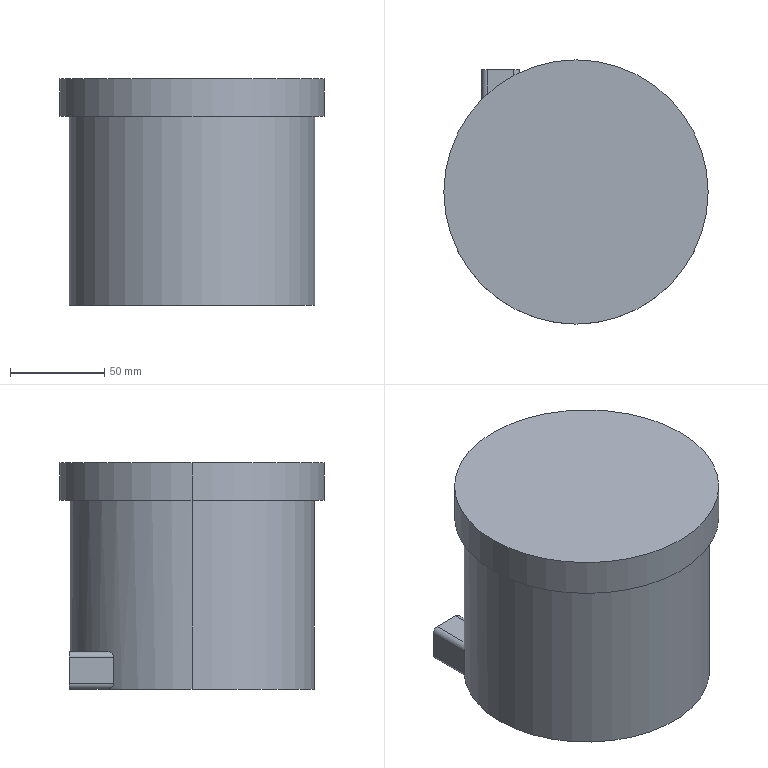Part | SolidWorks | features ICE 3, Extrusion 1, Fillet 1 | 1 solid | 18 faces | box 140 x 140 x 120 mm | volume 1639624 mm3 | cylinder 10 | plane 8 | commonest cylinder face diameters 6 x4 10 x2 130 x2 140 x2
STEP:
#1=CARTESIAN_POINT('',(-40.,50.,5.));
#2=VERTEX_POINT('',#1);
#3=CARTESIAN_POINT('',(-40.,50.,15.));
#4=VERTEX_POINT('',#3);
#5=CARTESIAN_POINT('',(-40.,50.,10.));
#6=DIRECTION('',(0.,1.,0.));
#7=DIRECTION('',(0.,0.,1.));
#8=AXIS2_PLACEMENT_3D('',#5,#6,#7);
#9=CIRCLE('',#8,5.);
#10=EDGE_CURVE('',#2,#4,#9,.T.);
#11=ORIENTED_EDGE('',*,*,#10,.F.);
#12=CARTESIAN_POINT('',(-40.,65.,5.));
#13=VERTEX_POINT('',#12);
#14=CARTESIAN_POINT('',(-40.,50.,5.));
#15=DIRECTION('',(0.,1.,0.));
#16=VECTOR('',#15,1000.);
#17=LINE('',#14,#16);
#18=EDGE_CURVE('',#2,#13,#17,.T.);
#19=ORIENTED_EDGE('',*,*,#18,.T.);
#20=CARTESIAN_POINT('',(-40.,65.,15.));
#21=VERTEX_POINT('',#20);
#22=CARTESIAN_POINT('',(-40.,65.,10.));
#23=DIRECTION('',(0.,1.,0.));
#24=DIRECTION('',(0.,0.,1.));
#25=AXIS2_PLACEMENT_3D('',#22,#23,#24);
#26=CIRCLE('',#25,5.);
#27=EDGE_CURVE('',#13,#21,#26,.T.);
#28=ORIENTED_EDGE('',*,*,#27,.T.);
#29=CARTESIAN_POINT('',(-40.,50.,15.));
#30=DIRECTION('',(0.,1.,0.));
#31=VECTOR('',#30,1000.);
#32=LINE('',#29,#31);
#33=EDGE_CURVE('',#4,#21,#32,.T.);
#34=ORIENTED_EDGE('',*,*,#33,.F.);
#35=EDGE_LOOP('',(#11,#19,#28,#34));
#36=FACE_OUTER_BOUND('',#35,.T.);
#37=CARTESIAN_POINT('',(-40.,50.,10.));
#38=DIRECTION('',(0.,1.,0.));
#39=DIRECTION('',(0.,0.,1.));
#40=AXIS2_PLACEMENT_3D('',#37,#38,#39);
#41=CYLINDRICAL_SURFACE('',#40,5.);
#42=ADVANCED_FACE('',(#36),#41,.F.);
#43=CARTESIAN_POINT('',(70.,0.,120.));
#44=VERTEX_POINT('',#43);
#45=CARTESIAN_POINT('',(-70.,0.,120.));
#46=VERTEX_POINT('',#45);
#47=CARTESIAN_POINT('',(0.,0.,120.));
#48=DIRECTION('',(0.,0.,1.));
#49=DIRECTION('',(1.,0.,0.));
#50=AXIS2_PLACEMENT_3D('',#47,#48,#49);
#51=CIRCLE('',#50,70.);
#52=EDGE_CURVE('',#44,#46,#51,.T.);
#53=ORIENTED_EDGE('',*,*,#52,.F.);
#54=CARTESIAN_POINT('',(70.,0.,100.));
#55=VERTEX_POINT('',#54);
#56=CARTESIAN_POINT('',(70.,0.,120.));
#57=DIRECTION('',(0.,0.,-1.));
#58=VECTOR('',#57,1000.);
#59=LINE('',#56,#58);
#60=EDGE_CURVE('',#44,#55,#59,.T.);
#61=ORIENTED_EDGE('',*,*,#60,.T.);
#62=CARTESIAN_POINT('',(-70.,0.,100.));
#63=VERTEX_POINT('',#62);
#64=CARTESIAN_POINT('',(0.,0.,100.));
#65=DIRECTION('',(0.,0.,1.));
#66=DIRECTION('',(1.,0.,0.));
#67=AXIS2_PLACEMENT_3D('',#64,#65,#66);
#68=CIRCLE('',#67,70.);
#69=EDGE_CURVE('',#55,#63,#68,.T.);
#70=ORIENTED_EDGE('',*,*,#69,.T.);
#71=CARTESIAN_POINT('',(-70.,0.,120.));
#72=DIRECTION('',(0.,0.,-1.));
#73=VECTOR('',#72,1000.);
#74=LINE('',#71,#73);
#75=EDGE_CURVE('',#46,#63,#74,.T.);
#76=ORIENTED_EDGE('',*,*,#75,.F.);
#77=EDGE_LOOP('',(#53,#61,#70,#76));
#78=FACE_OUTER_BOUND('',#77,.T.);
#79=CARTESIAN_POINT('',(0.,0.,120.));
#80=DIRECTION('',(0.,0.,-1.));
#81=DIRECTION('',(-1.,0.,0.));
#82=AXIS2_PLACEMENT_3D('',#79,#80,#81);
#83=CYLINDRICAL_SURFACE('',#82,70.);
#84=ADVANCED_FACE('',(#78),#83,.T.);
#85=CARTESIAN_POINT('',(65.,0.,100.));
#86=VERTEX_POINT('',#85);
#87=CARTESIAN_POINT('',(-65.,0.,100.));
#88=VERTEX_POINT('',#87);
#89=CARTESIAN_POINT('',(0.,0.,100.));
#90=DIRECTION('',(0.,0.,1.));
#91=DIRECTION('',(1.,0.,0.));
#92=AXIS2_PLACEMENT_3D('',#89,#90,#91);
#93=CIRCLE('',#92,65.);
#94=EDGE_CURVE('',#86,#88,#93,.T.);
#95=ORIENTED_EDGE('',*,*,#94,.F.);
#96=CARTESIAN_POINT('',(65.,0.,0.));
#97=VERTEX_POINT('',#96);
#98=CARTESIAN_POINT('',(65.,0.,100.));
#99=DIRECTION('',(0.,0.,-1.));
#100=VECTOR('',#99,1000.);
#101=LINE('',#98,#100);
#102=EDGE_CURVE('',#86,#97,#101,.T.);
#103=ORIENTED_EDGE('',*,*,#102,.T.);
#104=CARTESIAN_POINT('',(-33.,56.,0.));
#105=VERTEX_POINT('',#104);
#106=CARTESIAN_POINT('',(0.,0.,0.));
#107=DIRECTION('',(0.,0.,1.));
#108=DIRECTION('',(1.,0.,0.));
#109=AXIS2_PLACEMENT_3D('',#106,#107,#108);
#110=CIRCLE('',#109,65.);
#111=EDGE_CURVE('',#97,#105,#110,.T.);
#112=ORIENTED_EDGE('',*,*,#111,.T.);
#113=CARTESIAN_POINT('',(-30.,57.663,3.));
#114=VERTEX_POINT('',#113);
#115=CARTESIAN_POINT('',(-33.,56.,0.));
#116=CARTESIAN_POINT('',(-32.633,56.216,0.));
#117=CARTESIAN_POINT('',(-32.275,56.422,0.06519));
#118=CARTESIAN_POINT('',(-31.753,56.717,0.2653));
#119=CARTESIAN_POINT('',(-31.58,56.813,0.3504));
#120=CARTESIAN_POINT('',(-31.256,56.992,0.5513));
#121=CARTESIAN_POINT('',(-31.103,57.075,0.6674));
#122=CARTESIAN_POINT('',(-30.816,57.231,0.9335));
#123=CARTESIAN_POINT('',(-30.681,57.303,1.086));
#124=CARTESIAN_POINT('',(-30.447,57.428,1.412));
#125=CARTESIAN_POINT('',(-30.345,57.482,1.588));
#126=CARTESIAN_POINT('',(-30.176,57.571,1.966));
#127=CARTESIAN_POINT('',(-30.11,57.605,2.168));
#128=CARTESIAN_POINT('',(-30.023,57.651,2.577));
#129=CARTESIAN_POINT('',(-30.,57.663,2.786));
#130=CARTESIAN_POINT('',(-30.,57.663,3.));
#131=B_SPLINE_CURVE_WITH_KNOTS('',3,(#115,#116,#117,#118,#119,#120,#121,#122,#123,#124,#125,#126,#127,#128,#129,#130),.UNSPECIFIED.,.F.,.F.,(4,2,2,2,2,2,2,4),(0.,0.001254,0.001881,0.002508,0.003135,0.003762,0.004389,0.005016),.UNSPECIFIED.);
#132=EDGE_CURVE('',#105,#114,#131,.T.);
#133=ORIENTED_EDGE('',*,*,#132,.T.);
#134=CARTESIAN_POINT('',(-30.,57.663,17.));
#135=VERTEX_POINT('',#134);
#136=CARTESIAN_POINT('',(-30.,57.663,100.));
#137=DIRECTION('',(0.,0.,1.));
#138=VECTOR('',#137,1000.);
#139=LINE('',#136,#138);
#140=EDGE_CURVE('',#114,#135,#139,.T.);
#141=ORIENTED_EDGE('',*,*,#140,.T.);
#142=CARTESIAN_POINT('',(-33.,56.,20.));
#143=VERTEX_POINT('',#142);
#144=CARTESIAN_POINT('',(-30.,57.663,17.));
#145=CARTESIAN_POINT('',(-30.,57.663,17.213));
#146=CARTESIAN_POINT('',(-30.022,57.651,17.422));
#147=CARTESIAN_POINT('',(-30.11,57.606,17.83));
#148=CARTESIAN_POINT('',(-30.176,57.571,18.032));
#149=CARTESIAN_POINT('',(-30.343,57.483,18.408));
#150=CARTESIAN_POINT('',(-30.445,57.429,18.585));
#151=CARTESIAN_POINT('',(-30.681,57.303,18.914));
#152=CARTESIAN_POINT('',(-30.813,57.233,19.063));
#153=CARTESIAN_POINT('',(-31.099,57.078,19.329));
#154=CARTESIAN_POINT('',(-31.256,56.992,19.448));
#155=CARTESIAN_POINT('',(-31.579,56.814,19.649));
#156=CARTESIAN_POINT('',(-31.748,56.72,19.733));
#157=CARTESIAN_POINT('',(-32.098,56.522,19.867));
#158=CARTESIAN_POINT('',(-32.277,56.42,19.917));
#159=CARTESIAN_POINT('',(-32.636,56.213,19.983));
#160=CARTESIAN_POINT('',(-32.817,56.108,20.));
#161=CARTESIAN_POINT('',(-33.,56.,20.));
#162=B_SPLINE_CURVE_WITH_KNOTS('',3,(#144,#145,#146,#147,#148,#149,#150,#151,#152,#153,#154,#155,#156,#157,#158,#159,#160,#161),.UNSPECIFIED.,.F.,.F.,(4,2,2,2,2,2,2,2,4),(0.,0.0006295,0.001259,0.001888,0.002518,0.003147,0.003777,0.004406,0.005036),.UNSPECIFIED.);
#163=EDGE_CURVE('',#135,#143,#162,.T.);
#164=ORIENTED_EDGE('',*,*,#163,.T.);
#165=CARTESIAN_POINT('',(-47.,44.9,20.));
#166=VERTEX_POINT('',#165);
#167=CARTESIAN_POINT('',(0.,0.,20.));
#168=DIRECTION('',(0.,0.,1.));
#169=DIRECTION('',(1.,0.,0.));
#170=AXIS2_PLACEMENT_3D('',#167,#168,#169);
#171=CIRCLE('',#170,65.);
#172=EDGE_CURVE('',#143,#166,#171,.T.);
#173=ORIENTED_EDGE('',*,*,#172,.T.);
#174=CARTESIAN_POINT('',(-50.,41.533,17.));
#175=VERTEX_POINT('',#174);
#176=CARTESIAN_POINT('',(-47.,44.9,20.));
#177=CARTESIAN_POINT('',(-47.344,44.54,20.));
#178=CARTESIAN_POINT('',(-47.677,44.183,19.943));
#179=CARTESIAN_POINT('',(-48.322,43.477,19.715));
#180=CARTESIAN_POINT('',(-48.636,43.124,19.542));
#181=CARTESIAN_POINT('',(-49.063,42.636,19.186));
#182=CARTESIAN_POINT('',(-49.2,42.478,19.049));
#183=CARTESIAN_POINT('',(-49.453,42.183,18.738));
#184=CARTESIAN_POINT('',(-49.568,42.048,18.566));
#185=CARTESIAN_POINT('',(-49.768,41.811,18.177));
#186=CARTESIAN_POINT('',(-49.852,41.711,17.962));
#187=CARTESIAN_POINT('',(-49.939,41.607,17.615));
#188=CARTESIAN_POINT('',(-49.962,41.579,17.494));
#189=CARTESIAN_POINT('',(-49.992,41.543,17.249));
#190=CARTESIAN_POINT('',(-50.,41.533,17.126));
#191=CARTESIAN_POINT('',(-50.,41.533,17.));
#192=B_SPLINE_CURVE_WITH_KNOTS('',3,(#176,#177,#178,#179,#180,#181,#182,#183,#184,#185,#186,#187,#188,#189,#190,#191),.UNSPECIFIED.,.F.,.F.,(4,2,2,2,2,2,2,4),(0.,0.001472,0.002944,0.00368,0.004416,0.005152,0.00552,0.005888),.UNSPECIFIED.);
#193=EDGE_CURVE('',#166,#175,#192,.T.);
#194=ORIENTED_EDGE('',*,*,#193,.T.);
#195=CARTESIAN_POINT('',(-50.,41.533,3.));
#196=VERTEX_POINT('',#195);
#197=CARTESIAN_POINT('',(-50.,41.533,100.));
#198=DIRECTION('',(0.,0.,-1.));
#199=VECTOR('',#198,1000.);
#200=LINE('',#197,#199);
#201=EDGE_CURVE('',#175,#196,#200,.T.);
#202=ORIENTED_EDGE('',*,*,#201,.T.);
#203=CARTESIAN_POINT('',(-47.,44.9,0.));
#204=VERTEX_POINT('',#203);
#205=CARTESIAN_POINT('',(-50.,41.533,3.));
#206=CARTESIAN_POINT('',(-50.,41.533,2.749));
#207=CARTESIAN_POINT('',(-49.969,41.571,2.507));
#208=CARTESIAN_POINT('',(-49.852,41.71,2.04));
#209=CARTESIAN_POINT('',(-49.77,41.809,1.827));
#210=CARTESIAN_POINT('',(-49.569,42.046,1.436));
#211=CARTESIAN_POINT('',(-49.454,42.182,1.263));
#212=CARTESIAN_POINT('',(-49.203,42.474,0.9543));
#213=CARTESIAN_POINT('',(-49.066,42.633,0.8168));
#214=CARTESIAN_POINT('',(-48.638,43.122,0.4594));
#215=CARTESIAN_POINT('',(-48.33,43.468,0.2887));
#216=CARTESIAN_POINT('',(-47.678,44.182,0.05729));
#217=CARTESIAN_POINT('',(-47.344,44.54,0.));
#218=CARTESIAN_POINT('',(-47.,44.9,0.));
#219=B_SPLINE_CURVE_WITH_KNOTS('',3,(#205,#206,#207,#208,#209,#210,#211,#212,#213,#214,#215,#216,#217,#218),.UNSPECIFIED.,.F.,.F.,(4,2,2,2,2,2,4),(0.,0.0007398,0.00148,0.002219,0.002959,0.004439,0.005918),.UNSPECIFIED.);
#220=EDGE_CURVE('',#196,#204,#219,.T.);
#221=ORIENTED_EDGE('',*,*,#220,.T.);
#222=CARTESIAN_POINT('',(-65.,0.,0.));
#223=VERTEX_POINT('',#222);
#224=CARTESIAN_POINT('',(0.,0.,0.));
#225=DIRECTION('',(0.,0.,1.));
#226=DIRECTION('',(1.,0.,0.));
#227=AXIS2_PLACEMENT_3D('',#224,#225,#226);
#228=CIRCLE('',#227,65.);
#229=EDGE_CURVE('',#204,#223,#228,.T.);
#230=ORIENTED_EDGE('',*,*,#229,.T.);
#231=CARTESIAN_POINT('',(-65.,0.,100.));
#232=DIRECTION('',(0.,0.,-1.));
#233=VECTOR('',#232,1000.);
#234=LINE('',#231,#233);
#235=EDGE_CURVE('',#88,#223,#234,.T.);
#236=ORIENTED_EDGE('',*,*,#235,.F.);
#237=EDGE_LOOP('',(#95,#103,#112,#133,#141,#164,#173,#194,#202,#221,#230,#236));
#238=FACE_OUTER_BOUND('',#237,.T.);
#239=CARTESIAN_POINT('',(0.,0.,100.));
#240=DIRECTION('',(0.,0.,-1.));
#241=DIRECTION('',(-1.,0.,0.));
#242=AXIS2_PLACEMENT_3D('',#239,#240,#241);
#243=CYLINDRICAL_SURFACE('',#242,65.);
#244=ADVANCED_FACE('',(#238),#243,.T.);
#245=ORIENTED_EDGE('',*,*,#102,.F.);
#246=CARTESIAN_POINT('',(0.,0.,100.));
#247=DIRECTION('',(0.,0.,1.));
#248=DIRECTION('',(1.,0.,0.));
#249=AXIS2_PLACEMENT_3D('',#246,#247,#248);
#250=CIRCLE('',#249,65.);
#251=EDGE_CURVE('',#88,#86,#250,.T.);
#252=ORIENTED_EDGE('',*,*,#251,.F.);
#253=ORIENTED_EDGE('',*,*,#235,.T.);
#254=CARTESIAN_POINT('',(0.,0.,0.));
#255=DIRECTION('',(0.,0.,1.));
#256=DIRECTION('',(1.,0.,0.));
#257=AXIS2_PLACEMENT_3D('',#254,#255,#256);
#258=CIRCLE('',#257,65.);
#259=EDGE_CURVE('',#223,#97,#258,.T.);
#260=ORIENTED_EDGE('',*,*,#259,.T.);
#261=EDGE_LOOP('',(#245,#252,#253,#260));
#262=FACE_OUTER_BOUND('',#261,.T.);
#263=CARTESIAN_POINT('',(0.,0.,100.));
#264=DIRECTION('',(0.,0.,-1.));
#265=DIRECTION('',(-1.,0.,0.));
#266=AXIS2_PLACEMENT_3D('',#263,#264,#265);
#267=CYLINDRICAL_SURFACE('',#266,65.);
#268=ADVANCED_FACE('',(#262),#267,.T.);
#269=CARTESIAN_POINT('',(-47.,65.,0.));
#270=VERTEX_POINT('',#269);
#271=CARTESIAN_POINT('',(-33.,65.,0.));
#272=VERTEX_POINT('',#271);
#273=CARTESIAN_POINT('',(-30.,65.,0.));
#274=DIRECTION('',(1.,0.,0.));
#275=VECTOR('',#274,1000.);
#276=LINE('',#273,#275);
#277=EDGE_CURVE('',#270,#272,#276,.T.);
#278=ORIENTED_EDGE('',*,*,#277,.T.);
#279=CARTESIAN_POINT('',(-33.,57.663,0.));
#280=DIRECTION('',(0.,-1.,0.));
#281=VECTOR('',#280,1000.);
#282=LINE('',#279,#281);
#283=EDGE_CURVE('',#272,#105,#282,.T.);
#284=ORIENTED_EDGE('',*,*,#283,.T.);
#285=ORIENTED_EDGE('',*,*,#111,.F.);
#286=ORIENTED_EDGE('',*,*,#259,.F.);
#287=ORIENTED_EDGE('',*,*,#229,.F.);
#288=CARTESIAN_POINT('',(-47.,65.,0.));
#289=DIRECTION('',(0.,1.,0.));
#290=VECTOR('',#289,1000.);
#291=LINE('',#288,#290);
#292=EDGE_CURVE('',#204,#270,#291,.T.);
#293=ORIENTED_EDGE('',*,*,#292,.T.);
#294=EDGE_LOOP('',(#278,#284,#285,#286,#287,#293));
#295=FACE_OUTER_BOUND('',#294,.T.);
#296=CARTESIAN_POINT('',(0.,0.,0.));
#297=DIRECTION('',(0.,0.,1.));
#298=DIRECTION('',(1.,0.,0.));
#299=AXIS2_PLACEMENT_3D('',#296,#297,#298);
#300=PLANE('',#299);
#301=ADVANCED_FACE('',(#295),#300,.F.);
#302=ORIENTED_EDGE('',*,*,#60,.F.);
#303=CARTESIAN_POINT('',(0.,0.,120.));
#304=DIRECTION('',(0.,0.,1.));
#305=DIRECTION('',(1.,0.,0.));
#306=AXIS2_PLACEMENT_3D('',#303,#304,#305);
#307=CIRCLE('',#306,70.);
#308=EDGE_CURVE('',#46,#44,#307,.T.);
#309=ORIENTED_EDGE('',*,*,#308,.F.);
#310=ORIENTED_EDGE('',*,*,#75,.T.);
#311=CARTESIAN_POINT('',(0.,0.,100.));
#312=DIRECTION('',(0.,0.,1.));
#313=DIRECTION('',(1.,0.,0.));
#314=AXIS2_PLACEMENT_3D('',#311,#312,#313);
#315=CIRCLE('',#314,70.);
#316=EDGE_CURVE('',#63,#55,#315,.T.);
#317=ORIENTED_EDGE('',*,*,#316,.T.);
#318=EDGE_LOOP('',(#302,#309,#310,#317));
#319=FACE_OUTER_BOUND('',#318,.T.);
#320=CARTESIAN_POINT('',(0.,0.,120.));
#321=DIRECTION('',(0.,0.,-1.));
#322=DIRECTION('',(-1.,0.,0.));
#323=AXIS2_PLACEMENT_3D('',#320,#321,#322);
#324=CYLINDRICAL_SURFACE('',#323,70.);
#325=ADVANCED_FACE('',(#319),#324,.T.);
#326=ORIENTED_EDGE('',*,*,#308,.T.);
#327=ORIENTED_EDGE('',*,*,#52,.T.);
#328=EDGE_LOOP('',(#326,#327));
#329=FACE_OUTER_BOUND('',#328,.T.);
#330=CARTESIAN_POINT('',(0.,0.,120.));
#331=DIRECTION('',(0.,0.,1.));
#332=DIRECTION('',(1.,0.,0.));
#333=AXIS2_PLACEMENT_3D('',#330,#331,#332);
#334=PLANE('',#333);
#335=ADVANCED_FACE('',(#329),#334,.T.);
#336=ORIENTED_EDGE('',*,*,#251,.T.);
#337=ORIENTED_EDGE('',*,*,#94,.T.);
#338=EDGE_LOOP('',(#336,#337));
#339=FACE_BOUND('',#338,.T.);
#340=ORIENTED_EDGE('',*,*,#316,.F.);
#341=ORIENTED_EDGE('',*,*,#69,.F.);
#342=EDGE_LOOP('',(#340,#341));
#343=FACE_OUTER_BOUND('',#342,.T.);
#344=CARTESIAN_POINT('',(0.,0.,100.));
#345=DIRECTION('',(0.,0.,1.));
#346=DIRECTION('',(1.,0.,0.));
#347=AXIS2_PLACEMENT_3D('',#344,#345,#346);
#348=PLANE('',#347);
#349=ADVANCED_FACE('',(#339,#343),#348,.F.);
#350=ORIENTED_EDGE('',*,*,#140,.F.);
#351=CARTESIAN_POINT('',(-30.,65.,3.));
#352=VERTEX_POINT('',#351);
#353=CARTESIAN_POINT('',(-30.,65.,3.));
#354=DIRECTION('',(0.,1.,0.));
#355=VECTOR('',#354,1000.);
#356=LINE('',#353,#355);
#357=EDGE_CURVE('',#114,#352,#356,.T.);
#358=ORIENTED_EDGE('',*,*,#357,.T.);
#359=CARTESIAN_POINT('',(-30.,65.,17.));
#360=VERTEX_POINT('',#359);
#361=CARTESIAN_POINT('',(-30.,65.,20.));
#362=DIRECTION('',(0.,0.,-1.));
#363=VECTOR('',#362,1000.);
#364=LINE('',#361,#363);
#365=EDGE_CURVE('',#360,#352,#364,.T.);
#366=ORIENTED_EDGE('',*,*,#365,.F.);
#367=CARTESIAN_POINT('',(-30.,40.911,17.));
#368=DIRECTION('',(0.,-1.,0.));
#369=VECTOR('',#368,1000.);
#370=LINE('',#367,#369);
#371=EDGE_CURVE('',#360,#135,#370,.T.);
#372=ORIENTED_EDGE('',*,*,#371,.T.);
#373=EDGE_LOOP('',(#350,#358,#366,#372));
#374=FACE_OUTER_BOUND('',#373,.T.);
#375=CARTESIAN_POINT('',(-30.,40.911,20.));
#376=DIRECTION('',(1.,0.,0.));
#377=DIRECTION('',(0.,0.,-1.));
#378=AXIS2_PLACEMENT_3D('',#375,#376,#377);
#379=PLANE('',#378);
#380=ADVANCED_FACE('',(#374),#379,.T.);
#381=CARTESIAN_POINT('',(-50.,65.,17.));
#382=VERTEX_POINT('',#381);
#383=CARTESIAN_POINT('',(-50.,65.,3.));
#384=VERTEX_POINT('',#383);
#385=CARTESIAN_POINT('',(-50.,65.,20.));
#386=DIRECTION('',(0.,0.,-1.));
#387=VECTOR('',#386,1000.);
#388=LINE('',#385,#387);
#389=EDGE_CURVE('',#382,#384,#388,.T.);
#390=ORIENTED_EDGE('',*,*,#389,.T.);
#391=CARTESIAN_POINT('',(-50.,41.533,3.));
#392=DIRECTION('',(0.,-1.,0.));
#393=VECTOR('',#392,1000.);
#394=LINE('',#391,#393);
#395=EDGE_CURVE('',#384,#196,#394,.T.);
#396=ORIENTED_EDGE('',*,*,#395,.T.);
#397=ORIENTED_EDGE('',*,*,#201,.F.);
#398=CARTESIAN_POINT('',(-50.,40.911,17.));
#399=DIRECTION('',(0.,1.,0.));
#400=VECTOR('',#399,1000.);
#401=LINE('',#398,#400);
#402=EDGE_CURVE('',#175,#382,#401,.T.);
#403=ORIENTED_EDGE('',*,*,#402,.T.);
#404=EDGE_LOOP('',(#390,#396,#397,#403));
#405=FACE_OUTER_BOUND('',#404,.T.);
#406=CARTESIAN_POINT('',(-50.,40.911,20.));
#407=DIRECTION('',(-1.,0.,0.));
#408=DIRECTION('',(0.,0.,1.));
#409=AXIS2_PLACEMENT_3D('',#406,#407,#408);
#410=PLANE('',#409);
#411=ADVANCED_FACE('',(#405),#410,.T.);
#412=CARTESIAN_POINT('',(-40.,65.,10.));
#413=DIRECTION('',(0.,1.,0.));
#414=DIRECTION('',(0.,0.,1.));
#415=AXIS2_PLACEMENT_3D('',#412,#413,#414);
#416=CIRCLE('',#415,5.);
#417=EDGE_CURVE('',#21,#13,#416,.T.);
#418=ORIENTED_EDGE('',*,*,#417,.F.);
#419=ORIENTED_EDGE('',*,*,#27,.F.);
#420=EDGE_LOOP('',(#418,#419));
#421=FACE_BOUND('',#420,.T.);
#422=ORIENTED_EDGE('',*,*,#365,.T.);
#423=CARTESIAN_POINT('',(-33.,65.,3.));
#424=DIRECTION('',(0.,1.,0.));
#425=DIRECTION('',(0.,0.,1.));
#426=AXIS2_PLACEMENT_3D('',#423,#424,#425);
#427=CIRCLE('',#426,3.);
#428=EDGE_CURVE('',#352,#272,#427,.T.);
#429=ORIENTED_EDGE('',*,*,#428,.T.);
#430=ORIENTED_EDGE('',*,*,#277,.F.);
#431=CARTESIAN_POINT('',(-47.,65.,3.));
#432=DIRECTION('',(0.,1.,0.));
#433=DIRECTION('',(0.,0.,1.));
#434=AXIS2_PLACEMENT_3D('',#431,#432,#433);
#435=CIRCLE('',#434,3.);
#436=EDGE_CURVE('',#270,#384,#435,.T.);
#437=ORIENTED_EDGE('',*,*,#436,.T.);
#438=ORIENTED_EDGE('',*,*,#389,.F.);
#439=CARTESIAN_POINT('',(-47.,65.,20.));
#440=VERTEX_POINT('',#439);
#441=CARTESIAN_POINT('',(-47.,65.,17.));
#442=DIRECTION('',(0.,1.,0.));
#443=DIRECTION('',(0.,0.,1.));
#444=AXIS2_PLACEMENT_3D('',#441,#442,#443);
#445=CIRCLE('',#444,3.);
#446=EDGE_CURVE('',#382,#440,#445,.T.);
#447=ORIENTED_EDGE('',*,*,#446,.T.);
#448=CARTESIAN_POINT('',(-33.,65.,20.));
#449=VERTEX_POINT('',#448);
#450=CARTESIAN_POINT('',(-30.,65.,20.));
#451=DIRECTION('',(1.,0.,0.));
#452=VECTOR('',#451,1000.);
#453=LINE('',#450,#452);
#454=EDGE_CURVE('',#440,#449,#453,.T.);
#455=ORIENTED_EDGE('',*,*,#454,.T.);
#456=CARTESIAN_POINT('',(-33.,65.,17.));
#457=DIRECTION('',(0.,1.,0.));
#458=DIRECTION('',(0.,0.,1.));
#459=AXIS2_PLACEMENT_3D('',#456,#457,#458);
#460=CIRCLE('',#459,3.);
#461=EDGE_CURVE('',#449,#360,#460,.T.);
#462=ORIENTED_EDGE('',*,*,#461,.T.);
#463=EDGE_LOOP('',(#422,#429,#430,#437,#438,#447,#455,#462));
#464=FACE_OUTER_BOUND('',#463,.T.);
#465=CARTESIAN_POINT('',(-30.,65.,20.));
#466=DIRECTION('',(0.,1.,0.));
#467=DIRECTION('',(0.,0.,1.));
#468=AXIS2_PLACEMENT_3D('',#465,#466,#467);
#469=PLANE('',#468);
#470=ADVANCED_FACE('',(#421,#464),#469,.T.);
#471=ORIENTED_EDGE('',*,*,#172,.F.);
#472=CARTESIAN_POINT('',(-33.,0.,20.));
#473=DIRECTION('',(0.,1.,0.));
#474=VECTOR('',#473,1000.);
#475=LINE('',#472,#474);
#476=EDGE_CURVE('',#143,#449,#475,.T.);
#477=ORIENTED_EDGE('',*,*,#476,.T.);
#478=ORIENTED_EDGE('',*,*,#454,.F.);
#479=CARTESIAN_POINT('',(-47.,0.,20.));
#480=DIRECTION('',(0.,-1.,0.));
#481=VECTOR('',#480,1000.);
#482=LINE('',#479,#481);
#483=EDGE_CURVE('',#440,#166,#482,.T.);
#484=ORIENTED_EDGE('',*,*,#483,.T.);
#485=EDGE_LOOP('',(#471,#477,#478,#484));
#486=FACE_OUTER_BOUND('',#485,.T.);
#487=CARTESIAN_POINT('',(0.,0.,20.));
#488=DIRECTION('',(0.,0.,1.));
#489=DIRECTION('',(1.,0.,0.));
#490=AXIS2_PLACEMENT_3D('',#487,#488,#489);
#491=PLANE('',#490);
#492=ADVANCED_FACE('',(#486),#491,.T.);
#493=ORIENTED_EDGE('',*,*,#18,.F.);
#494=CARTESIAN_POINT('',(-40.,50.,10.));
#495=DIRECTION('',(0.,1.,0.));
#496=DIRECTION('',(0.,0.,1.));
#497=AXIS2_PLACEMENT_3D('',#494,#495,#496);
#498=CIRCLE('',#497,5.);
#499=EDGE_CURVE('',#4,#2,#498,.T.);
#500=ORIENTED_EDGE('',*,*,#499,.F.);
#501=ORIENTED_EDGE('',*,*,#33,.T.);
#502=ORIENTED_EDGE('',*,*,#417,.T.);
#503=EDGE_LOOP('',(#493,#500,#501,#502));
#504=FACE_OUTER_BOUND('',#503,.T.);
#505=CARTESIAN_POINT('',(-40.,50.,10.));
#506=DIRECTION('',(0.,1.,0.));
#507=DIRECTION('',(0.,0.,1.));
#508=AXIS2_PLACEMENT_3D('',#505,#506,#507);
#509=CYLINDRICAL_SURFACE('',#508,5.);
#510=ADVANCED_FACE('',(#504),#509,.F.);
#511=ORIENTED_EDGE('',*,*,#499,.T.);
#512=ORIENTED_EDGE('',*,*,#10,.T.);
#513=EDGE_LOOP('',(#511,#512));
#514=FACE_OUTER_BOUND('',#513,.T.);
#515=CARTESIAN_POINT('',(-40.,50.,10.));
#516=DIRECTION('',(0.,1.,0.));
#517=DIRECTION('',(0.,0.,1.));
#518=AXIS2_PLACEMENT_3D('',#515,#516,#517);
#519=PLANE('',#518);
#520=ADVANCED_FACE('',(#514),#519,.T.);
#521=ORIENTED_EDGE('',*,*,#428,.F.);
#522=ORIENTED_EDGE('',*,*,#357,.F.);
#523=ORIENTED_EDGE('',*,*,#132,.F.);
#524=ORIENTED_EDGE('',*,*,#283,.F.);
#525=EDGE_LOOP('',(#521,#522,#523,#524));
#526=FACE_OUTER_BOUND('',#525,.T.);
#527=CARTESIAN_POINT('',(-33.,0.,3.));
#528=DIRECTION('',(0.,1.,0.));
#529=DIRECTION('',(0.,0.,1.));
#530=AXIS2_PLACEMENT_3D('',#527,#528,#529);
#531=CYLINDRICAL_SURFACE('',#530,3.);
#532=ADVANCED_FACE('',(#526),#531,.T.);
#533=ORIENTED_EDGE('',*,*,#461,.F.);
#534=ORIENTED_EDGE('',*,*,#476,.F.);
#535=ORIENTED_EDGE('',*,*,#163,.F.);
#536=ORIENTED_EDGE('',*,*,#371,.F.);
#537=EDGE_LOOP('',(#533,#534,#535,#536));
#538=FACE_OUTER_BOUND('',#537,.T.);
#539=CARTESIAN_POINT('',(-33.,40.911,17.));
#540=DIRECTION('',(0.,-1.,0.));
#541=DIRECTION('',(0.,0.,-1.));
#542=AXIS2_PLACEMENT_3D('',#539,#540,#541);
#543=CYLINDRICAL_SURFACE('',#542,3.);
#544=ADVANCED_FACE('',(#538),#543,.T.);
#545=ORIENTED_EDGE('',*,*,#220,.F.);
#546=ORIENTED_EDGE('',*,*,#395,.F.);
#547=ORIENTED_EDGE('',*,*,#436,.F.);
#548=ORIENTED_EDGE('',*,*,#292,.F.);
#549=EDGE_LOOP('',(#545,#546,#547,#548));
#550=FACE_OUTER_BOUND('',#549,.T.);
#551=CARTESIAN_POINT('',(-47.,0.,3.));
#552=DIRECTION('',(0.,-1.,0.));
#553=DIRECTION('',(0.,0.,-1.));
#554=AXIS2_PLACEMENT_3D('',#551,#552,#553);
#555=CYLINDRICAL_SURFACE('',#554,3.);
#556=ADVANCED_FACE('',(#550),#555,.T.);
#557=ORIENTED_EDGE('',*,*,#193,.F.);
#558=ORIENTED_EDGE('',*,*,#483,.F.);
#559=ORIENTED_EDGE('',*,*,#446,.F.);
#560=ORIENTED_EDGE('',*,*,#402,.F.);
#561=EDGE_LOOP('',(#557,#558,#559,#560));
#562=FACE_OUTER_BOUND('',#561,.T.);
#563=CARTESIAN_POINT('',(-47.,40.911,17.));
#564=DIRECTION('',(0.,1.,0.));
#565=DIRECTION('',(0.,0.,1.));
#566=AXIS2_PLACEMENT_3D('',#563,#564,#565);
#567=CYLINDRICAL_SURFACE('',#566,3.);
#568=ADVANCED_FACE('',(#562),#567,.T.);
#569=CLOSED_SHELL('',(#42,#84,#244,#268,#301,#325,#335,#349,#380,#411,#470,#492,#510,#520,#532,#544,#556,#568));
#570=MANIFOLD_SOLID_BREP('',#569);
#571=CARTESIAN_POINT('',(0.,0.,0.));
#572=DIRECTION('',(0.,0.,1.));
#573=DIRECTION('',(1.,0.,0.));
#574=AXIS2_PLACEMENT_3D('',#571,#572,#573);
#575=(LENGTH_UNIT()NAMED_UNIT(*)SI_UNIT(.MILLI.,.METRE.));
#576=UNCERTAINTY_MEASURE_WITH_UNIT(LENGTH_MEASURE(0.00001),#575,'','');
#577=(NAMED_UNIT(*)PLANE_ANGLE_UNIT()SI_UNIT($,.RADIAN.));
#578=(NAMED_UNIT(*)SI_UNIT($,.STERADIAN.)SOLID_ANGLE_UNIT());
#579=(GEOMETRIC_REPRESENTATION_CONTEXT(3)GLOBAL_UNCERTAINTY_ASSIGNED_CONTEXT((#576))GLOBAL_UNIT_ASSIGNED_CONTEXT((#575,#577,#578))REPRESENTATION_CONTEXT('',''));
#580=ADVANCED_BREP_SHAPE_REPRESENTATION('',(#570,#574),#579);